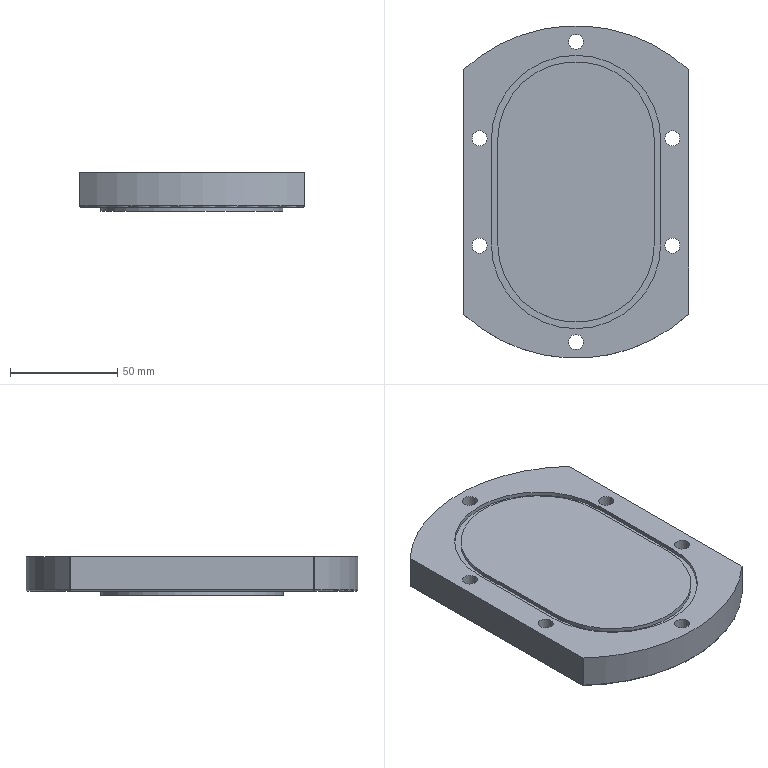Part | 1 solid | 52 faces | box 105 x 155 x 18 mm | volume 242328 mm3 | cylinder 24 | plane 17 | cone 6 | sphere 3 | torus 2 | commonest cylinder face diameters 7 x6 11 x6 1 x5 73 x2 79 x2 155 x2
STEP:
#1=CARTESIAN_POINT('',(52.5,-57.009,0.));
#2=VERTEX_POINT('',#1);
#3=CARTESIAN_POINT('',(-52.338,-57.158,0.));
#4=VERTEX_POINT('',#3);
#5=CARTESIAN_POINT('',(0.,0.,0.));
#6=DIRECTION('',(0.,0.,-1.));
#7=DIRECTION('',(-1.,0.,0.));
#8=AXIS2_PLACEMENT_3D('',#5,#6,#7);
#9=CIRCLE('',#8,77.5);
#10=EDGE_CURVE('',#2,#4,#9,.T.);
#11=ORIENTED_EDGE('',*,*,#10,.T.);
#12=CARTESIAN_POINT('',(-52.338,-57.158,-15.5));
#13=VERTEX_POINT('',#12);
#14=CARTESIAN_POINT('',(-52.338,-57.158,-16.));
#15=DIRECTION('',(0.,0.,1.));
#16=VECTOR('',#15,1000.);
#17=LINE('',#14,#16);
#18=EDGE_CURVE('',#4,#13,#17,.F.);
#19=ORIENTED_EDGE('',*,*,#18,.T.);
#20=CARTESIAN_POINT('',(52.5,-57.009,-15.5));
#21=VERTEX_POINT('',#20);
#22=CARTESIAN_POINT('',(0.,0.,-15.5));
#23=DIRECTION('',(0.,0.,-1.));
#24=DIRECTION('',(-1.,0.,0.));
#25=AXIS2_PLACEMENT_3D('',#22,#23,#24);
#26=CIRCLE('',#25,77.5);
#27=EDGE_CURVE('',#13,#21,#26,.F.);
#28=ORIENTED_EDGE('',*,*,#27,.T.);
#29=CARTESIAN_POINT('',(52.5,-57.009,-16.));
#30=DIRECTION('',(0.,0.,1.));
#31=VECTOR('',#30,1000.);
#32=LINE('',#29,#31);
#33=EDGE_CURVE('',#21,#2,#32,.T.);
#34=ORIENTED_EDGE('',*,*,#33,.T.);
#35=EDGE_LOOP('',(#11,#19,#28,#34));
#36=FACE_BOUND('',#35,.T.);
#37=CARTESIAN_POINT('',(0.,0.,-16.));
#38=DIRECTION('',(0.,0.,1.));
#39=DIRECTION('',(1.,0.,0.));
#40=AXIS2_PLACEMENT_3D('',#37,#38,#39);
#41=CYLINDRICAL_SURFACE('',#40,77.5);
#42=ADVANCED_FACE('',(#36),#41,.T.);
#43=CARTESIAN_POINT('',(-52.5,-56.789,0.));
#44=VERTEX_POINT('',#43);
#45=CARTESIAN_POINT('',(-52.5,56.789,0.));
#46=VERTEX_POINT('',#45);
#47=CARTESIAN_POINT('',(-52.5,-57.009,0.));
#48=DIRECTION('',(0.,1.,0.));
#49=VECTOR('',#48,1000.);
#50=LINE('',#47,#49);
#51=EDGE_CURVE('',#44,#46,#50,.T.);
#52=ORIENTED_EDGE('',*,*,#51,.T.);
#53=CARTESIAN_POINT('',(-52.5,56.789,-15.5));
#54=VERTEX_POINT('',#53);
#55=CARTESIAN_POINT('',(-52.5,56.789,-16.));
#56=DIRECTION('',(0.,0.,1.));
#57=VECTOR('',#56,1000.);
#58=LINE('',#55,#57);
#59=EDGE_CURVE('',#46,#54,#58,.F.);
#60=ORIENTED_EDGE('',*,*,#59,.T.);
#61=CARTESIAN_POINT('',(-52.5,-56.789,-15.5));
#62=VERTEX_POINT('',#61);
#63=CARTESIAN_POINT('',(-52.5,-57.009,-15.5));
#64=DIRECTION('',(0.,1.,0.));
#65=VECTOR('',#64,1000.);
#66=LINE('',#63,#65);
#67=EDGE_CURVE('',#54,#62,#66,.F.);
#68=ORIENTED_EDGE('',*,*,#67,.T.);
#69=CARTESIAN_POINT('',(-52.5,-56.789,-16.));
#70=DIRECTION('',(0.,0.,1.));
#71=VECTOR('',#70,1000.);
#72=LINE('',#69,#71);
#73=EDGE_CURVE('',#62,#44,#72,.T.);
#74=ORIENTED_EDGE('',*,*,#73,.T.);
#75=EDGE_LOOP('',(#52,#60,#68,#74));
#76=FACE_BOUND('',#75,.T.);
#77=CARTESIAN_POINT('',(-52.5,-57.009,-16.));
#78=DIRECTION('',(1.,0.,0.));
#79=DIRECTION('',(0.,0.,-1.));
#80=AXIS2_PLACEMENT_3D('',#77,#78,#79);
#81=PLANE('',#80);
#82=ADVANCED_FACE('',(#76),#81,.F.);
#83=CARTESIAN_POINT('',(-52.338,57.158,0.));
#84=VERTEX_POINT('',#83);
#85=CARTESIAN_POINT('',(52.338,57.158,0.));
#86=VERTEX_POINT('',#85);
#87=CARTESIAN_POINT('',(0.,0.,0.));
#88=DIRECTION('',(0.,0.,-1.));
#89=DIRECTION('',(-1.,0.,0.));
#90=AXIS2_PLACEMENT_3D('',#87,#88,#89);
#91=CIRCLE('',#90,77.5);
#92=EDGE_CURVE('',#84,#86,#91,.T.);
#93=ORIENTED_EDGE('',*,*,#92,.T.);
#94=CARTESIAN_POINT('',(52.338,57.158,-15.5));
#95=VERTEX_POINT('',#94);
#96=CARTESIAN_POINT('',(52.338,57.158,-16.));
#97=DIRECTION('',(0.,0.,1.));
#98=VECTOR('',#97,1000.);
#99=LINE('',#96,#98);
#100=EDGE_CURVE('',#86,#95,#99,.F.);
#101=ORIENTED_EDGE('',*,*,#100,.T.);
#102=CARTESIAN_POINT('',(-52.338,57.158,-15.5));
#103=VERTEX_POINT('',#102);
#104=CARTESIAN_POINT('',(0.,0.,-15.5));
#105=DIRECTION('',(0.,0.,-1.));
#106=DIRECTION('',(-1.,0.,0.));
#107=AXIS2_PLACEMENT_3D('',#104,#105,#106);
#108=CIRCLE('',#107,77.5);
#109=EDGE_CURVE('',#95,#103,#108,.F.);
#110=ORIENTED_EDGE('',*,*,#109,.T.);
#111=CARTESIAN_POINT('',(-52.338,57.158,-16.));
#112=DIRECTION('',(0.,0.,1.));
#113=VECTOR('',#112,1000.);
#114=LINE('',#111,#113);
#115=EDGE_CURVE('',#103,#84,#114,.T.);
#116=ORIENTED_EDGE('',*,*,#115,.T.);
#117=EDGE_LOOP('',(#93,#101,#110,#116));
#118=FACE_BOUND('',#117,.T.);
#119=CARTESIAN_POINT('',(0.,0.,-16.));
#120=DIRECTION('',(0.,0.,1.));
#121=DIRECTION('',(1.,0.,0.));
#122=AXIS2_PLACEMENT_3D('',#119,#120,#121);
#123=CYLINDRICAL_SURFACE('',#122,77.5);
#124=ADVANCED_FACE('',(#118),#123,.T.);
#125=CARTESIAN_POINT('',(52.5,56.789,-15.5));
#126=VERTEX_POINT('',#125);
#127=CARTESIAN_POINT('',(52.5,57.009,-15.5));
#128=DIRECTION('',(0.,-1.,0.));
#129=VECTOR('',#128,1000.);
#130=LINE('',#127,#129);
#131=EDGE_CURVE('',#21,#126,#130,.F.);
#132=ORIENTED_EDGE('',*,*,#131,.T.);
#133=CARTESIAN_POINT('',(52.5,56.789,0.));
#134=VERTEX_POINT('',#133);
#135=CARTESIAN_POINT('',(52.5,56.789,-16.));
#136=DIRECTION('',(0.,0.,1.));
#137=VECTOR('',#136,1000.);
#138=LINE('',#135,#137);
#139=EDGE_CURVE('',#126,#134,#138,.T.);
#140=ORIENTED_EDGE('',*,*,#139,.T.);
#141=CARTESIAN_POINT('',(52.5,57.009,0.));
#142=DIRECTION('',(0.,-1.,0.));
#143=VECTOR('',#142,1000.);
#144=LINE('',#141,#143);
#145=EDGE_CURVE('',#134,#2,#144,.T.);
#146=ORIENTED_EDGE('',*,*,#145,.T.);
#147=ORIENTED_EDGE('',*,*,#33,.F.);
#148=EDGE_LOOP('',(#132,#140,#146,#147));
#149=FACE_BOUND('',#148,.T.);
#150=CARTESIAN_POINT('',(52.5,57.009,-16.));
#151=DIRECTION('',(-1.,0.,0.));
#152=DIRECTION('',(0.,0.,1.));
#153=AXIS2_PLACEMENT_3D('',#150,#151,#152);
#154=PLANE('',#153);
#155=ADVANCED_FACE('',(#149),#154,.F.);
#156=CARTESIAN_POINT('',(-52.,-56.789,-16.));
#157=VERTEX_POINT('',#156);
#158=CARTESIAN_POINT('',(-52.,56.789,-16.));
#159=VERTEX_POINT('',#158);
#160=CARTESIAN_POINT('',(-52.,57.009,-16.));
#161=DIRECTION('',(0.,1.,0.));
#162=VECTOR('',#161,1000.);
#163=LINE('',#160,#162);
#164=EDGE_CURVE('',#157,#159,#163,.T.);
#165=ORIENTED_EDGE('',*,*,#164,.T.);
#166=CARTESIAN_POINT('',(52.,56.789,-16.));
#167=VERTEX_POINT('',#166);
#168=CARTESIAN_POINT('',(0.,0.,-16.));
#169=DIRECTION('',(0.,0.,-1.));
#170=DIRECTION('',(-1.,0.,0.));
#171=AXIS2_PLACEMENT_3D('',#168,#169,#170);
#172=CIRCLE('',#171,77.);
#173=EDGE_CURVE('',#159,#167,#172,.T.);
#174=ORIENTED_EDGE('',*,*,#173,.T.);
#175=CARTESIAN_POINT('',(52.,-56.789,-16.));
#176=VERTEX_POINT('',#175);
#177=CARTESIAN_POINT('',(52.,-57.009,-16.));
#178=DIRECTION('',(0.,-1.,0.));
#179=VECTOR('',#178,1000.);
#180=LINE('',#177,#179);
#181=EDGE_CURVE('',#167,#176,#180,.T.);
#182=ORIENTED_EDGE('',*,*,#181,.T.);
#183=CARTESIAN_POINT('',(0.,0.,-16.));
#184=DIRECTION('',(0.,0.,-1.));
#185=DIRECTION('',(-1.,0.,0.));
#186=AXIS2_PLACEMENT_3D('',#183,#184,#185);
#187=CIRCLE('',#186,77.);
#188=EDGE_CURVE('',#176,#157,#187,.T.);
#189=ORIENTED_EDGE('',*,*,#188,.T.);
#190=EDGE_LOOP('',(#165,#174,#182,#189));
#191=FACE_BOUND('',#190,.T.);
#192=CARTESIAN_POINT('',(-5.525,70.,-16.));
#193=VERTEX_POINT('',#192);
#194=CARTESIAN_POINT('',(0.,70.,-16.));
#195=DIRECTION('',(0.,0.,-1.));
#196=DIRECTION('',(-1.,0.,0.));
#197=AXIS2_PLACEMENT_3D('',#194,#195,#196);
#198=CIRCLE('',#197,5.525);
#199=EDGE_CURVE('',#193,#193,#198,.T.);
#200=ORIENTED_EDGE('',*,*,#199,.F.);
#201=EDGE_LOOP('',(#200));
#202=FACE_BOUND('',#201,.T.);
#203=CARTESIAN_POINT('',(39.475,25.,-16.));
#204=VERTEX_POINT('',#203);
#205=CARTESIAN_POINT('',(45.,25.,-16.));
#206=DIRECTION('',(0.,0.,-1.));
#207=DIRECTION('',(-1.,0.,0.));
#208=AXIS2_PLACEMENT_3D('',#205,#206,#207);
#209=CIRCLE('',#208,5.525);
#210=EDGE_CURVE('',#204,#204,#209,.T.);
#211=ORIENTED_EDGE('',*,*,#210,.F.);
#212=EDGE_LOOP('',(#211));
#213=FACE_BOUND('',#212,.T.);
#214=CARTESIAN_POINT('',(-50.525,25.,-16.));
#215=VERTEX_POINT('',#214);
#216=CARTESIAN_POINT('',(-45.,25.,-16.));
#217=DIRECTION('',(0.,0.,-1.));
#218=DIRECTION('',(-1.,0.,0.));
#219=AXIS2_PLACEMENT_3D('',#216,#217,#218);
#220=CIRCLE('',#219,5.525);
#221=EDGE_CURVE('',#215,#215,#220,.T.);
#222=ORIENTED_EDGE('',*,*,#221,.F.);
#223=EDGE_LOOP('',(#222));
#224=FACE_BOUND('',#223,.T.);
#225=CARTESIAN_POINT('',(-50.525,-25.,-16.));
#226=VERTEX_POINT('',#225);
#227=CARTESIAN_POINT('',(-45.,-25.,-16.));
#228=DIRECTION('',(0.,0.,-1.));
#229=DIRECTION('',(-1.,0.,0.));
#230=AXIS2_PLACEMENT_3D('',#227,#228,#229);
#231=CIRCLE('',#230,5.525);
#232=EDGE_CURVE('',#226,#226,#231,.T.);
#233=ORIENTED_EDGE('',*,*,#232,.F.);
#234=EDGE_LOOP('',(#233));
#235=FACE_BOUND('',#234,.T.);
#236=CARTESIAN_POINT('',(39.475,-25.,-16.));
#237=VERTEX_POINT('',#236);
#238=CARTESIAN_POINT('',(45.,-25.,-16.));
#239=DIRECTION('',(0.,0.,-1.));
#240=DIRECTION('',(-1.,0.,0.));
#241=AXIS2_PLACEMENT_3D('',#238,#239,#240);
#242=CIRCLE('',#241,5.525);
#243=EDGE_CURVE('',#237,#237,#242,.T.);
#244=ORIENTED_EDGE('',*,*,#243,.F.);
#245=EDGE_LOOP('',(#244));
#246=FACE_BOUND('',#245,.T.);
#247=CARTESIAN_POINT('',(-5.525,-70.,-16.));
#248=VERTEX_POINT('',#247);
#249=CARTESIAN_POINT('',(0.,-70.,-16.));
#250=DIRECTION('',(0.,0.,-1.));
#251=DIRECTION('',(-1.,0.,0.));
#252=AXIS2_PLACEMENT_3D('',#249,#250,#251);
#253=CIRCLE('',#252,5.525);
#254=EDGE_CURVE('',#248,#248,#253,.T.);
#255=ORIENTED_EDGE('',*,*,#254,.F.);
#256=EDGE_LOOP('',(#255));
#257=FACE_BOUND('',#256,.T.);
#258=CARTESIAN_POINT('',(-42.5,0.,-16.));
#259=VERTEX_POINT('',#258);
#260=CARTESIAN_POINT('',(0.,0.,-16.));
#261=DIRECTION('',(0.,0.,-1.));
#262=DIRECTION('',(-1.,0.,0.));
#263=AXIS2_PLACEMENT_3D('',#260,#261,#262);
#264=CIRCLE('',#263,42.5);
#265=EDGE_CURVE('',#259,#259,#264,.T.);
#266=ORIENTED_EDGE('',*,*,#265,.F.);
#267=EDGE_LOOP('',(#266));
#268=FACE_BOUND('',#267,.T.);
#269=CARTESIAN_POINT('',(0.,0.,-16.));
#270=DIRECTION('',(0.,0.,-1.));
#271=DIRECTION('',(-1.,0.,0.));
#272=AXIS2_PLACEMENT_3D('',#269,#270,#271);
#273=PLANE('',#272);
#274=ADVANCED_FACE('',(#191,#202,#213,#224,#235,#246,#257,#268),#273,.T.);
#275=CARTESIAN_POINT('',(-39.5,24.25,0.));
#276=VERTEX_POINT('',#275);
#277=CARTESIAN_POINT('',(-39.5,-24.25,0.));
#278=VERTEX_POINT('',#277);
#279=CARTESIAN_POINT('',(-39.5,24.25,0.));
#280=DIRECTION('',(0.,-1.,0.));
#281=VECTOR('',#280,1000.);
#282=LINE('',#279,#281);
#283=EDGE_CURVE('',#276,#278,#282,.T.);
#284=ORIENTED_EDGE('',*,*,#283,.F.);
#285=CARTESIAN_POINT('',(39.5,24.25,0.));
#286=VERTEX_POINT('',#285);
#287=CARTESIAN_POINT('',(0.,24.25,0.));
#288=DIRECTION('',(0.,0.,1.));
#289=DIRECTION('',(1.,0.,0.));
#290=AXIS2_PLACEMENT_3D('',#287,#288,#289);
#291=CIRCLE('',#290,39.5);
#292=EDGE_CURVE('',#286,#276,#291,.T.);
#293=ORIENTED_EDGE('',*,*,#292,.F.);
#294=CARTESIAN_POINT('',(39.5,-24.25,0.));
#295=VERTEX_POINT('',#294);
#296=CARTESIAN_POINT('',(39.5,24.25,0.));
#297=DIRECTION('',(0.,1.,0.));
#298=VECTOR('',#297,1000.);
#299=LINE('',#296,#298);
#300=EDGE_CURVE('',#295,#286,#299,.T.);
#301=ORIENTED_EDGE('',*,*,#300,.F.);
#302=CARTESIAN_POINT('',(0.,-24.25,0.));
#303=DIRECTION('',(0.,0.,1.));
#304=DIRECTION('',(1.,0.,0.));
#305=AXIS2_PLACEMENT_3D('',#302,#303,#304);
#306=CIRCLE('',#305,39.5);
#307=EDGE_CURVE('',#278,#295,#306,.T.);
#308=ORIENTED_EDGE('',*,*,#307,.F.);
#309=EDGE_LOOP('',(#284,#293,#301,#308));
#310=FACE_BOUND('',#309,.T.);
#311=CARTESIAN_POINT('',(-3.5,70.,0.));
#312=VERTEX_POINT('',#311);
#313=CARTESIAN_POINT('',(0.,70.,0.));
#314=DIRECTION('',(0.,0.,-1.));
#315=DIRECTION('',(-1.,0.,0.));
#316=AXIS2_PLACEMENT_3D('',#313,#314,#315);
#317=CIRCLE('',#316,3.5);
#318=EDGE_CURVE('',#312,#312,#317,.T.);
#319=ORIENTED_EDGE('',*,*,#318,.T.);
#320=EDGE_LOOP('',(#319));
#321=FACE_BOUND('',#320,.T.);
#322=CARTESIAN_POINT('',(41.5,25.,0.));
#323=VERTEX_POINT('',#322);
#324=CARTESIAN_POINT('',(45.,25.,0.));
#325=DIRECTION('',(0.,0.,-1.));
#326=DIRECTION('',(-1.,0.,0.));
#327=AXIS2_PLACEMENT_3D('',#324,#325,#326);
#328=CIRCLE('',#327,3.5);
#329=EDGE_CURVE('',#323,#323,#328,.T.);
#330=ORIENTED_EDGE('',*,*,#329,.T.);
#331=EDGE_LOOP('',(#330));
#332=FACE_BOUND('',#331,.T.);
#333=CARTESIAN_POINT('',(-48.5,25.,0.));
#334=VERTEX_POINT('',#333);
#335=CARTESIAN_POINT('',(-45.,25.,0.));
#336=DIRECTION('',(0.,0.,-1.));
#337=DIRECTION('',(-1.,0.,0.));
#338=AXIS2_PLACEMENT_3D('',#335,#336,#337);
#339=CIRCLE('',#338,3.5);
#340=EDGE_CURVE('',#334,#334,#339,.T.);
#341=ORIENTED_EDGE('',*,*,#340,.T.);
#342=EDGE_LOOP('',(#341));
#343=FACE_BOUND('',#342,.T.);
#344=CARTESIAN_POINT('',(-48.5,-25.,0.));
#345=VERTEX_POINT('',#344);
#346=CARTESIAN_POINT('',(-45.,-25.,0.));
#347=DIRECTION('',(0.,0.,-1.));
#348=DIRECTION('',(-1.,0.,0.));
#349=AXIS2_PLACEMENT_3D('',#346,#347,#348);
#350=CIRCLE('',#349,3.5);
#351=EDGE_CURVE('',#345,#345,#350,.T.);
#352=ORIENTED_EDGE('',*,*,#351,.T.);
#353=EDGE_LOOP('',(#352));
#354=FACE_BOUND('',#353,.T.);
#355=CARTESIAN_POINT('',(41.5,-25.,0.));
#356=VERTEX_POINT('',#355);
#357=CARTESIAN_POINT('',(45.,-25.,0.));
#358=DIRECTION('',(0.,0.,-1.));
#359=DIRECTION('',(-1.,0.,0.));
#360=AXIS2_PLACEMENT_3D('',#357,#358,#359);
#361=CIRCLE('',#360,3.5);
#362=EDGE_CURVE('',#356,#356,#361,.T.);
#363=ORIENTED_EDGE('',*,*,#362,.T.);
#364=EDGE_LOOP('',(#363));
#365=FACE_BOUND('',#364,.T.);
#366=CARTESIAN_POINT('',(-3.5,-70.,0.));
#367=VERTEX_POINT('',#366);
#368=CARTESIAN_POINT('',(0.,-70.,0.));
#369=DIRECTION('',(0.,0.,-1.));
#370=DIRECTION('',(-1.,0.,0.));
#371=AXIS2_PLACEMENT_3D('',#368,#369,#370);
#372=CIRCLE('',#371,3.5);
#373=EDGE_CURVE('',#367,#367,#372,.T.);
#374=ORIENTED_EDGE('',*,*,#373,.T.);
#375=EDGE_LOOP('',(#374));
#376=FACE_BOUND('',#375,.T.);
#377=ORIENTED_EDGE('',*,*,#145,.F.);
#378=CARTESIAN_POINT('',(52.,56.789,0.));
#379=DIRECTION('',(0.,0.,-1.));
#380=DIRECTION('',(-1.,0.,0.));
#381=AXIS2_PLACEMENT_3D('',#378,#379,#380);
#382=CIRCLE('',#381,0.5);
#383=EDGE_CURVE('',#134,#86,#382,.F.);
#384=ORIENTED_EDGE('',*,*,#383,.T.);
#385=ORIENTED_EDGE('',*,*,#92,.F.);
#386=CARTESIAN_POINT('',(-52.,56.789,0.));
#387=DIRECTION('',(0.,0.,-1.));
#388=DIRECTION('',(-1.,0.,0.));
#389=AXIS2_PLACEMENT_3D('',#386,#387,#388);
#390=CIRCLE('',#389,0.5);
#391=EDGE_CURVE('',#84,#46,#390,.F.);
#392=ORIENTED_EDGE('',*,*,#391,.T.);
#393=ORIENTED_EDGE('',*,*,#51,.F.);
#394=CARTESIAN_POINT('',(-52.,-56.789,0.));
#395=DIRECTION('',(0.,0.,-1.));
#396=DIRECTION('',(-1.,0.,0.));
#397=AXIS2_PLACEMENT_3D('',#394,#395,#396);
#398=CIRCLE('',#397,0.5);
#399=EDGE_CURVE('',#44,#4,#398,.F.);
#400=ORIENTED_EDGE('',*,*,#399,.T.);
#401=ORIENTED_EDGE('',*,*,#10,.F.);
#402=EDGE_LOOP('',(#377,#384,#385,#392,#393,#400,#401));
#403=FACE_BOUND('',#402,.T.);
#404=CARTESIAN_POINT('',(0.,0.,0.));
#405=DIRECTION('',(0.,0.,-1.));
#406=DIRECTION('',(-1.,0.,0.));
#407=AXIS2_PLACEMENT_3D('',#404,#405,#406);
#408=PLANE('',#407);
#409=ADVANCED_FACE('',(#310,#321,#332,#343,#354,#365,#376,#403),#408,.F.);
#410=CARTESIAN_POINT('',(-42.5,0.,-18.));
#411=VERTEX_POINT('',#410);
#412=CARTESIAN_POINT('',(0.,0.,-18.));
#413=DIRECTION('',(0.,0.,-1.));
#414=DIRECTION('',(-1.,0.,0.));
#415=AXIS2_PLACEMENT_3D('',#412,#413,#414);
#416=CIRCLE('',#415,42.5);
#417=EDGE_CURVE('',#411,#411,#416,.T.);
#418=ORIENTED_EDGE('',*,*,#417,.F.);
#419=EDGE_LOOP('',(#418));
#420=FACE_BOUND('',#419,.T.);
#421=ORIENTED_EDGE('',*,*,#265,.T.);
#422=EDGE_LOOP('',(#421));
#423=FACE_BOUND('',#422,.T.);
#424=CARTESIAN_POINT('',(0.,0.,-18.));
#425=DIRECTION('',(0.,0.,1.));
#426=DIRECTION('',(1.,0.,0.));
#427=AXIS2_PLACEMENT_3D('',#424,#425,#426);
#428=CYLINDRICAL_SURFACE('',#427,42.5);
#429=ADVANCED_FACE('',(#420,#423),#428,.T.);
#430=ORIENTED_EDGE('',*,*,#417,.T.);
#431=EDGE_LOOP('',(#430));
#432=FACE_BOUND('',#431,.T.);
#433=CARTESIAN_POINT('',(0.,0.,-18.));
#434=DIRECTION('',(0.,0.,-1.));
#435=DIRECTION('',(-1.,0.,0.));
#436=AXIS2_PLACEMENT_3D('',#433,#434,#435);
#437=PLANE('',#436);
#438=ADVANCED_FACE('',(#432),#437,.T.);
#439=CARTESIAN_POINT('',(-3.5,-70.,-9.2));
#440=VERTEX_POINT('',#439);
#441=CARTESIAN_POINT('',(0.,-70.,-9.2));
#442=DIRECTION('',(0.,0.,-1.));
#443=DIRECTION('',(-1.,0.,0.));
#444=AXIS2_PLACEMENT_3D('',#441,#442,#443);
#445=CIRCLE('',#444,3.5);
#446=EDGE_CURVE('',#440,#440,#445,.T.);
#447=ORIENTED_EDGE('',*,*,#446,.T.);
#448=EDGE_LOOP('',(#447));
#449=FACE_BOUND('',#448,.T.);
#450=ORIENTED_EDGE('',*,*,#373,.F.);
#451=EDGE_LOOP('',(#450));
#452=FACE_BOUND('',#451,.T.);
#453=CARTESIAN_POINT('',(0.,-70.,-16.));
#454=DIRECTION('',(0.,0.,-1.));
#455=DIRECTION('',(-1.,0.,0.));
#456=AXIS2_PLACEMENT_3D('',#453,#454,#455);
#457=CYLINDRICAL_SURFACE('',#456,3.5);
#458=ADVANCED_FACE('',(#449,#452),#457,.F.);
#459=ORIENTED_EDGE('',*,*,#446,.F.);
#460=EDGE_LOOP('',(#459));
#461=FACE_BOUND('',#460,.T.);
#462=CARTESIAN_POINT('',(-5.5,-70.,-9.2));
#463=VERTEX_POINT('',#462);
#464=CARTESIAN_POINT('',(0.,-70.,-9.2));
#465=DIRECTION('',(0.,0.,-1.));
#466=DIRECTION('',(-1.,0.,0.));
#467=AXIS2_PLACEMENT_3D('',#464,#465,#466);
#468=CIRCLE('',#467,5.5);
#469=EDGE_CURVE('',#463,#463,#468,.T.);
#470=ORIENTED_EDGE('',*,*,#469,.T.);
#471=EDGE_LOOP('',(#470));
#472=FACE_BOUND('',#471,.T.);
#473=CARTESIAN_POINT('',(-3.5,-70.,-9.2));
#474=DIRECTION('',(0.,0.,1.));
#475=DIRECTION('',(1.,0.,0.));
#476=AXIS2_PLACEMENT_3D('',#473,#474,#475);
#477=PLANE('',#476);
#478=ADVANCED_FACE('',(#461,#472),#477,.F.);
#479=ORIENTED_EDGE('',*,*,#469,.F.);
#480=EDGE_LOOP('',(#479));
#481=FACE_BOUND('',#480,.T.);
#482=CARTESIAN_POINT('',(-5.5,-70.,-15.975));
#483=VERTEX_POINT('',#482);
#484=CARTESIAN_POINT('',(0.,-70.,-15.975));
#485=DIRECTION('',(0.,0.,-1.));
#486=DIRECTION('',(-1.,0.,0.));
#487=AXIS2_PLACEMENT_3D('',#484,#485,#486);
#488=CIRCLE('',#487,5.5);
#489=EDGE_CURVE('',#483,#483,#488,.T.);
#490=ORIENTED_EDGE('',*,*,#489,.T.);
#491=EDGE_LOOP('',(#490));
#492=FACE_BOUND('',#491,.T.);
#493=CARTESIAN_POINT('',(0.,-70.,-16.));
#494=DIRECTION('',(0.,0.,-1.));
#495=DIRECTION('',(-1.,0.,0.));
#496=AXIS2_PLACEMENT_3D('',#493,#494,#495);
#497=CYLINDRICAL_SURFACE('',#496,5.5);
#498=ADVANCED_FACE('',(#481,#492),#497,.F.);
#499=ORIENTED_EDGE('',*,*,#489,.F.);
#500=EDGE_LOOP('',(#499));
#501=FACE_BOUND('',#500,.T.);
#502=ORIENTED_EDGE('',*,*,#254,.T.);
#503=EDGE_LOOP('',(#502));
#504=FACE_BOUND('',#503,.T.);
#505=CARTESIAN_POINT('',(0.,-70.,-16.));
#506=DIRECTION('',(0.,0.,-1.));
#507=DIRECTION('',(-1.,0.,0.));
#508=AXIS2_PLACEMENT_3D('',#505,#506,#507);
#509=CONICAL_SURFACE('',#508,5.525,0.7854);
#510=ADVANCED_FACE('',(#501,#504),#509,.F.);
#511=CARTESIAN_POINT('',(41.5,-25.,-9.2));
#512=VERTEX_POINT('',#511);
#513=CARTESIAN_POINT('',(45.,-25.,-9.2));
#514=DIRECTION('',(0.,0.,-1.));
#515=DIRECTION('',(-1.,0.,0.));
#516=AXIS2_PLACEMENT_3D('',#513,#514,#515);
#517=CIRCLE('',#516,3.5);
#518=EDGE_CURVE('',#512,#512,#517,.T.);
#519=ORIENTED_EDGE('',*,*,#518,.T.);
#520=EDGE_LOOP('',(#519));
#521=FACE_BOUND('',#520,.T.);
#522=ORIENTED_EDGE('',*,*,#362,.F.);
#523=EDGE_LOOP('',(#522));
#524=FACE_BOUND('',#523,.T.);
#525=CARTESIAN_POINT('',(45.,-25.,-16.));
#526=DIRECTION('',(0.,0.,-1.));
#527=DIRECTION('',(-1.,0.,0.));
#528=AXIS2_PLACEMENT_3D('',#525,#526,#527);
#529=CYLINDRICAL_SURFACE('',#528,3.5);
#530=ADVANCED_FACE('',(#521,#524),#529,.F.);
#531=ORIENTED_EDGE('',*,*,#518,.F.);
#532=EDGE_LOOP('',(#531));
#533=FACE_BOUND('',#532,.T.);
#534=CARTESIAN_POINT('',(39.5,-25.,-9.2));
#535=VERTEX_POINT('',#534);
#536=CARTESIAN_POINT('',(45.,-25.,-9.2));
#537=DIRECTION('',(0.,0.,-1.));
#538=DIRECTION('',(-1.,0.,0.));
#539=AXIS2_PLACEMENT_3D('',#536,#537,#538);
#540=CIRCLE('',#539,5.5);
#541=EDGE_CURVE('',#535,#535,#540,.T.);
#542=ORIENTED_EDGE('',*,*,#541,.T.);
#543=EDGE_LOOP('',(#542));
#544=FACE_BOUND('',#543,.T.);
#545=CARTESIAN_POINT('',(41.5,-25.,-9.2));
#546=DIRECTION('',(0.,0.,1.));
#547=DIRECTION('',(1.,0.,0.));
#548=AXIS2_PLACEMENT_3D('',#545,#546,#547);
#549=PLANE('',#548);
#550=ADVANCED_FACE('',(#533,#544),#549,.F.);
#551=ORIENTED_EDGE('',*,*,#541,.F.);
#552=EDGE_LOOP('',(#551));
#553=FACE_BOUND('',#552,.T.);
#554=CARTESIAN_POINT('',(39.5,-25.,-15.975));
#555=VERTEX_POINT('',#554);
#556=CARTESIAN_POINT('',(45.,-25.,-15.975));
#557=DIRECTION('',(0.,0.,-1.));
#558=DIRECTION('',(-1.,0.,0.));
#559=AXIS2_PLACEMENT_3D('',#556,#557,#558);
#560=CIRCLE('',#559,5.5);
#561=EDGE_CURVE('',#555,#555,#560,.T.);
#562=ORIENTED_EDGE('',*,*,#561,.T.);
#563=EDGE_LOOP('',(#562));
#564=FACE_BOUND('',#563,.T.);
#565=CARTESIAN_POINT('',(45.,-25.,-16.));
#566=DIRECTION('',(0.,0.,-1.));
#567=DIRECTION('',(-1.,0.,0.));
#568=AXIS2_PLACEMENT_3D('',#565,#566,#567);
#569=CYLINDRICAL_SURFACE('',#568,5.5);
#570=ADVANCED_FACE('',(#553,#564),#569,.F.);
#571=ORIENTED_EDGE('',*,*,#561,.F.);
#572=EDGE_LOOP('',(#571));
#573=FACE_BOUND('',#572,.T.);
#574=ORIENTED_EDGE('',*,*,#243,.T.);
#575=EDGE_LOOP('',(#574));
#576=FACE_BOUND('',#575,.T.);
#577=CARTESIAN_POINT('',(45.,-25.,-16.));
#578=DIRECTION('',(0.,0.,-1.));
#579=DIRECTION('',(-1.,0.,0.));
#580=AXIS2_PLACEMENT_3D('',#577,#578,#579);
#581=CONICAL_SURFACE('',#580,5.525,0.7854);
#582=ADVANCED_FACE('',(#573,#576),#581,.F.);
#583=CARTESIAN_POINT('',(-48.5,-25.,-9.2));
#584=VERTEX_POINT('',#583);
#585=CARTESIAN_POINT('',(-45.,-25.,-9.2));
#586=DIRECTION('',(0.,0.,-1.));
#587=DIRECTION('',(-1.,0.,0.));
#588=AXIS2_PLACEMENT_3D('',#585,#586,#587);
#589=CIRCLE('',#588,3.5);
#590=EDGE_CURVE('',#584,#584,#589,.T.);
#591=ORIENTED_EDGE('',*,*,#590,.T.);
#592=EDGE_LOOP('',(#591));
#593=FACE_BOUND('',#592,.T.);
#594=ORIENTED_EDGE('',*,*,#351,.F.);
#595=EDGE_LOOP('',(#594));
#596=FACE_BOUND('',#595,.T.);
#597=CARTESIAN_POINT('',(-45.,-25.,-16.));
#598=DIRECTION('',(0.,0.,-1.));
#599=DIRECTION('',(-1.,0.,0.));
#600=AXIS2_PLACEMENT_3D('',#597,#598,#599);
#601=CYLINDRICAL_SURFACE('',#600,3.5);
#602=ADVANCED_FACE('',(#593,#596),#601,.F.);
#603=ORIENTED_EDGE('',*,*,#590,.F.);
#604=EDGE_LOOP('',(#603));
#605=FACE_BOUND('',#604,.T.);
#606=CARTESIAN_POINT('',(-50.5,-25.,-9.2));
#607=VERTEX_POINT('',#606);
#608=CARTESIAN_POINT('',(-45.,-25.,-9.2));
#609=DIRECTION('',(0.,0.,-1.));
#610=DIRECTION('',(-1.,0.,0.));
#611=AXIS2_PLACEMENT_3D('',#608,#609,#610);
#612=CIRCLE('',#611,5.5);
#613=EDGE_CURVE('',#607,#607,#612,.T.);
#614=ORIENTED_EDGE('',*,*,#613,.T.);
#615=EDGE_LOOP('',(#614));
#616=FACE_BOUND('',#615,.T.);
#617=CARTESIAN_POINT('',(-48.5,-25.,-9.2));
#618=DIRECTION('',(0.,0.,1.));
#619=DIRECTION('',(1.,0.,0.));
#620=AXIS2_PLACEMENT_3D('',#617,#618,#619);
#621=PLANE('',#620);
#622=ADVANCED_FACE('',(#605,#616),#621,.F.);
#623=ORIENTED_EDGE('',*,*,#613,.F.);
#624=EDGE_LOOP('',(#623));
#625=FACE_BOUND('',#624,.T.);
#626=CARTESIAN_POINT('',(-50.5,-25.,-15.975));
#627=VERTEX_POINT('',#626);
#628=CARTESIAN_POINT('',(-45.,-25.,-15.975));
#629=DIRECTION('',(0.,0.,-1.));
#630=DIRECTION('',(-1.,0.,0.));
#631=AXIS2_PLACEMENT_3D('',#628,#629,#630);
#632=CIRCLE('',#631,5.5);
#633=EDGE_CURVE('',#627,#627,#632,.T.);
#634=ORIENTED_EDGE('',*,*,#633,.T.);
#635=EDGE_LOOP('',(#634));
#636=FACE_BOUND('',#635,.T.);
#637=CARTESIAN_POINT('',(-45.,-25.,-16.));
#638=DIRECTION('',(0.,0.,-1.));
#639=DIRECTION('',(-1.,0.,0.));
#640=AXIS2_PLACEMENT_3D('',#637,#638,#639);
#641=CYLINDRICAL_SURFACE('',#640,5.5);
#642=ADVANCED_FACE('',(#625,#636),#641,.F.);
#643=ORIENTED_EDGE('',*,*,#633,.F.);
#644=EDGE_LOOP('',(#643));
#645=FACE_BOUND('',#644,.T.);
#646=ORIENTED_EDGE('',*,*,#232,.T.);
#647=EDGE_LOOP('',(#646));
#648=FACE_BOUND('',#647,.T.);
#649=CARTESIAN_POINT('',(-45.,-25.,-16.));
#650=DIRECTION('',(0.,0.,-1.));
#651=DIRECTION('',(-1.,0.,0.));
#652=AXIS2_PLACEMENT_3D('',#649,#650,#651);
#653=CONICAL_SURFACE('',#652,5.525,0.7854);
#654=ADVANCED_FACE('',(#645,#648),#653,.F.);
#655=CARTESIAN_POINT('',(-48.5,25.,-9.2));
#656=VERTEX_POINT('',#655);
#657=CARTESIAN_POINT('',(-45.,25.,-9.2));
#658=DIRECTION('',(0.,0.,-1.));
#659=DIRECTION('',(-1.,0.,0.));
#660=AXIS2_PLACEMENT_3D('',#657,#658,#659);
#661=CIRCLE('',#660,3.5);
#662=EDGE_CURVE('',#656,#656,#661,.T.);
#663=ORIENTED_EDGE('',*,*,#662,.T.);
#664=EDGE_LOOP('',(#663));
#665=FACE_BOUND('',#664,.T.);
#666=ORIENTED_EDGE('',*,*,#340,.F.);
#667=EDGE_LOOP('',(#666));
#668=FACE_BOUND('',#667,.T.);
#669=CARTESIAN_POINT('',(-45.,25.,-16.));
#670=DIRECTION('',(0.,0.,-1.));
#671=DIRECTION('',(-1.,0.,0.));
#672=AXIS2_PLACEMENT_3D('',#669,#670,#671);
#673=CYLINDRICAL_SURFACE('',#672,3.5);
#674=ADVANCED_FACE('',(#665,#668),#673,.F.);
#675=ORIENTED_EDGE('',*,*,#662,.F.);
#676=EDGE_LOOP('',(#675));
#677=FACE_BOUND('',#676,.T.);
#678=CARTESIAN_POINT('',(-50.5,25.,-9.2));
#679=VERTEX_POINT('',#678);
#680=CARTESIAN_POINT('',(-45.,25.,-9.2));
#681=DIRECTION('',(0.,0.,-1.));
#682=DIRECTION('',(-1.,0.,0.));
#683=AXIS2_PLACEMENT_3D('',#680,#681,#682);
#684=CIRCLE('',#683,5.5);
#685=EDGE_CURVE('',#679,#679,#684,.T.);
#686=ORIENTED_EDGE('',*,*,#685,.T.);
#687=EDGE_LOOP('',(#686));
#688=FACE_BOUND('',#687,.T.);
#689=CARTESIAN_POINT('',(-48.5,25.,-9.2));
#690=DIRECTION('',(0.,0.,1.));
#691=DIRECTION('',(1.,0.,0.));
#692=AXIS2_PLACEMENT_3D('',#689,#690,#691);
#693=PLANE('',#692);
#694=ADVANCED_FACE('',(#677,#688),#693,.F.);
#695=ORIENTED_EDGE('',*,*,#685,.F.);
#696=EDGE_LOOP('',(#695));
#697=FACE_BOUND('',#696,.T.);
#698=CARTESIAN_POINT('',(-50.5,25.,-15.975));
#699=VERTEX_POINT('',#698);
#700=CARTESIAN_POINT('',(-45.,25.,-15.975));
#701=DIRECTION('',(0.,0.,-1.));
#702=DIRECTION('',(-1.,0.,0.));
#703=AXIS2_PLACEMENT_3D('',#700,#701,#702);
#704=CIRCLE('',#703,5.5);
#705=EDGE_CURVE('',#699,#699,#704,.T.);
#706=ORIENTED_EDGE('',*,*,#705,.T.);
#707=EDGE_LOOP('',(#706));
#708=FACE_BOUND('',#707,.T.);
#709=CARTESIAN_POINT('',(-45.,25.,-16.));
#710=DIRECTION('',(0.,0.,-1.));
#711=DIRECTION('',(-1.,0.,0.));
#712=AXIS2_PLACEMENT_3D('',#709,#710,#711);
#713=CYLINDRICAL_SURFACE('',#712,5.5);
#714=ADVANCED_FACE('',(#697,#708),#713,.F.);
#715=ORIENTED_EDGE('',*,*,#705,.F.);
#716=EDGE_LOOP('',(#715));
#717=FACE_BOUND('',#716,.T.);
#718=ORIENTED_EDGE('',*,*,#221,.T.);
#719=EDGE_LOOP('',(#718));
#720=FACE_BOUND('',#719,.T.);
#721=CARTESIAN_POINT('',(-45.,25.,-16.));
#722=DIRECTION('',(0.,0.,-1.));
#723=DIRECTION('',(-1.,0.,0.));
#724=AXIS2_PLACEMENT_3D('',#721,#722,#723);
#725=CONICAL_SURFACE('',#724,5.525,0.7854);
#726=ADVANCED_FACE('',(#717,#720),#725,.F.);
#727=CARTESIAN_POINT('',(41.5,25.,-9.2));
#728=VERTEX_POINT('',#727);
#729=CARTESIAN_POINT('',(45.,25.,-9.2));
#730=DIRECTION('',(0.,0.,-1.));
#731=DIRECTION('',(-1.,0.,0.));
#732=AXIS2_PLACEMENT_3D('',#729,#730,#731);
#733=CIRCLE('',#732,3.5);
#734=EDGE_CURVE('',#728,#728,#733,.T.);
#735=ORIENTED_EDGE('',*,*,#734,.T.);
#736=EDGE_LOOP('',(#735));
#737=FACE_BOUND('',#736,.T.);
#738=ORIENTED_EDGE('',*,*,#329,.F.);
#739=EDGE_LOOP('',(#738));
#740=FACE_BOUND('',#739,.T.);
#741=CARTESIAN_POINT('',(45.,25.,-16.));
#742=DIRECTION('',(0.,0.,-1.));
#743=DIRECTION('',(-1.,0.,0.));
#744=AXIS2_PLACEMENT_3D('',#741,#742,#743);
#745=CYLINDRICAL_SURFACE('',#744,3.5);
#746=ADVANCED_FACE('',(#737,#740),#745,.F.);
#747=ORIENTED_EDGE('',*,*,#734,.F.);
#748=EDGE_LOOP('',(#747));
#749=FACE_BOUND('',#748,.T.);
#750=CARTESIAN_POINT('',(39.5,25.,-9.2));
#751=VERTEX_POINT('',#750);
#752=CARTESIAN_POINT('',(45.,25.,-9.2));
#753=DIRECTION('',(0.,0.,-1.));
#754=DIRECTION('',(-1.,0.,0.));
#755=AXIS2_PLACEMENT_3D('',#752,#753,#754);
#756=CIRCLE('',#755,5.5);
#757=EDGE_CURVE('',#751,#751,#756,.T.);
#758=ORIENTED_EDGE('',*,*,#757,.T.);
#759=EDGE_LOOP('',(#758));
#760=FACE_BOUND('',#759,.T.);
#761=CARTESIAN_POINT('',(41.5,25.,-9.2));
#762=DIRECTION('',(0.,0.,1.));
#763=DIRECTION('',(1.,0.,0.));
#764=AXIS2_PLACEMENT_3D('',#761,#762,#763);
#765=PLANE('',#764);
#766=ADVANCED_FACE('',(#749,#760),#765,.F.);
#767=ORIENTED_EDGE('',*,*,#757,.F.);
#768=EDGE_LOOP('',(#767));
#769=FACE_BOUND('',#768,.T.);
#770=CARTESIAN_POINT('',(39.5,25.,-15.975));
#771=VERTEX_POINT('',#770);
#772=CARTESIAN_POINT('',(45.,25.,-15.975));
#773=DIRECTION('',(0.,0.,-1.));
#774=DIRECTION('',(-1.,0.,0.));
#775=AXIS2_PLACEMENT_3D('',#772,#773,#774);
#776=CIRCLE('',#775,5.5);
#777=EDGE_CURVE('',#771,#771,#776,.T.);
#778=ORIENTED_EDGE('',*,*,#777,.T.);
#779=EDGE_LOOP('',(#778));
#780=FACE_BOUND('',#779,.T.);
#781=CARTESIAN_POINT('',(45.,25.,-16.));
#782=DIRECTION('',(0.,0.,-1.));
#783=DIRECTION('',(-1.,0.,0.));
#784=AXIS2_PLACEMENT_3D('',#781,#782,#783);
#785=CYLINDRICAL_SURFACE('',#784,5.5);
#786=ADVANCED_FACE('',(#769,#780),#785,.F.);
#787=ORIENTED_EDGE('',*,*,#777,.F.);
#788=EDGE_LOOP('',(#787));
#789=FACE_BOUND('',#788,.T.);
#790=ORIENTED_EDGE('',*,*,#210,.T.);
#791=EDGE_LOOP('',(#790));
#792=FACE_BOUND('',#791,.T.);
#793=CARTESIAN_POINT('',(45.,25.,-16.));
#794=DIRECTION('',(0.,0.,-1.));
#795=DIRECTION('',(-1.,0.,0.));
#796=AXIS2_PLACEMENT_3D('',#793,#794,#795);
#797=CONICAL_SURFACE('',#796,5.525,0.7854);
#798=ADVANCED_FACE('',(#789,#792),#797,.F.);
#799=CARTESIAN_POINT('',(-3.5,70.,-9.2));
#800=VERTEX_POINT('',#799);
#801=CARTESIAN_POINT('',(0.,70.,-9.2));
#802=DIRECTION('',(0.,0.,-1.));
#803=DIRECTION('',(-1.,0.,0.));
#804=AXIS2_PLACEMENT_3D('',#801,#802,#803);
#805=CIRCLE('',#804,3.5);
#806=EDGE_CURVE('',#800,#800,#805,.T.);
#807=ORIENTED_EDGE('',*,*,#806,.T.);
#808=EDGE_LOOP('',(#807));
#809=FACE_BOUND('',#808,.T.);
#810=ORIENTED_EDGE('',*,*,#318,.F.);
#811=EDGE_LOOP('',(#810));
#812=FACE_BOUND('',#811,.T.);
#813=CARTESIAN_POINT('',(0.,70.,-16.));
#814=DIRECTION('',(0.,0.,-1.));
#815=DIRECTION('',(-1.,0.,0.));
#816=AXIS2_PLACEMENT_3D('',#813,#814,#815);
#817=CYLINDRICAL_SURFACE('',#816,3.5);
#818=ADVANCED_FACE('',(#809,#812),#817,.F.);
#819=ORIENTED_EDGE('',*,*,#806,.F.);
#820=EDGE_LOOP('',(#819));
#821=FACE_BOUND('',#820,.T.);
#822=CARTESIAN_POINT('',(-5.5,70.,-9.2));
#823=VERTEX_POINT('',#822);
#824=CARTESIAN_POINT('',(0.,70.,-9.2));
#825=DIRECTION('',(0.,0.,-1.));
#826=DIRECTION('',(-1.,0.,0.));
#827=AXIS2_PLACEMENT_3D('',#824,#825,#826);
#828=CIRCLE('',#827,5.5);
#829=EDGE_CURVE('',#823,#823,#828,.T.);
#830=ORIENTED_EDGE('',*,*,#829,.T.);
#831=EDGE_LOOP('',(#830));
#832=FACE_BOUND('',#831,.T.);
#833=CARTESIAN_POINT('',(-3.5,70.,-9.2));
#834=DIRECTION('',(0.,0.,1.));
#835=DIRECTION('',(1.,0.,0.));
#836=AXIS2_PLACEMENT_3D('',#833,#834,#835);
#837=PLANE('',#836);
#838=ADVANCED_FACE('',(#821,#832),#837,.F.);
#839=ORIENTED_EDGE('',*,*,#829,.F.);
#840=EDGE_LOOP('',(#839));
#841=FACE_BOUND('',#840,.T.);
#842=CARTESIAN_POINT('',(-5.5,70.,-15.975));
#843=VERTEX_POINT('',#842);
#844=CARTESIAN_POINT('',(0.,70.,-15.975));
#845=DIRECTION('',(0.,0.,-1.));
#846=DIRECTION('',(-1.,0.,0.));
#847=AXIS2_PLACEMENT_3D('',#844,#845,#846);
#848=CIRCLE('',#847,5.5);
#849=EDGE_CURVE('',#843,#843,#848,.T.);
#850=ORIENTED_EDGE('',*,*,#849,.T.);
#851=EDGE_LOOP('',(#850));
#852=FACE_BOUND('',#851,.T.);
#853=CARTESIAN_POINT('',(0.,70.,-16.));
#854=DIRECTION('',(0.,0.,-1.));
#855=DIRECTION('',(-1.,0.,0.));
#856=AXIS2_PLACEMENT_3D('',#853,#854,#855);
#857=CYLINDRICAL_SURFACE('',#856,5.5);
#858=ADVANCED_FACE('',(#841,#852),#857,.F.);
#859=ORIENTED_EDGE('',*,*,#849,.F.);
#860=EDGE_LOOP('',(#859));
#861=FACE_BOUND('',#860,.T.);
#862=ORIENTED_EDGE('',*,*,#199,.T.);
#863=EDGE_LOOP('',(#862));
#864=FACE_BOUND('',#863,.T.);
#865=CARTESIAN_POINT('',(0.,70.,-16.));
#866=DIRECTION('',(0.,0.,-1.));
#867=DIRECTION('',(-1.,0.,0.));
#868=AXIS2_PLACEMENT_3D('',#865,#866,#867);
#869=CONICAL_SURFACE('',#868,5.525,0.7854);
#870=ADVANCED_FACE('',(#861,#864),#869,.F.);
#871=ORIENTED_EDGE('',*,*,#399,.F.);
#872=ORIENTED_EDGE('',*,*,#73,.F.);
#873=CARTESIAN_POINT('',(-52.,-56.789,-15.5));
#874=DIRECTION('',(0.,0.,-1.));
#875=DIRECTION('',(-1.,0.,0.));
#876=AXIS2_PLACEMENT_3D('',#873,#874,#875);
#877=CIRCLE('',#876,0.5);
#878=EDGE_CURVE('',#13,#62,#877,.T.);
#879=ORIENTED_EDGE('',*,*,#878,.F.);
#880=ORIENTED_EDGE('',*,*,#18,.F.);
#881=EDGE_LOOP('',(#871,#872,#879,#880));
#882=FACE_BOUND('',#881,.T.);
#883=CARTESIAN_POINT('',(-52.,-56.789,-16.));
#884=DIRECTION('',(0.,0.,1.));
#885=DIRECTION('',(1.,0.,0.));
#886=AXIS2_PLACEMENT_3D('',#883,#884,#885);
#887=CYLINDRICAL_SURFACE('',#886,0.5);
#888=ADVANCED_FACE('',(#882),#887,.T.);
#889=ORIENTED_EDGE('',*,*,#391,.F.);
#890=ORIENTED_EDGE('',*,*,#115,.F.);
#891=CARTESIAN_POINT('',(-52.,56.789,-15.5));
#892=DIRECTION('',(0.,0.,-1.));
#893=DIRECTION('',(-1.,0.,0.));
#894=AXIS2_PLACEMENT_3D('',#891,#892,#893);
#895=CIRCLE('',#894,0.5);
#896=EDGE_CURVE('',#54,#103,#895,.T.);
#897=ORIENTED_EDGE('',*,*,#896,.F.);
#898=ORIENTED_EDGE('',*,*,#59,.F.);
#899=EDGE_LOOP('',(#889,#890,#897,#898));
#900=FACE_BOUND('',#899,.T.);
#901=CARTESIAN_POINT('',(-52.,56.789,-16.));
#902=DIRECTION('',(0.,0.,1.));
#903=DIRECTION('',(1.,0.,0.));
#904=AXIS2_PLACEMENT_3D('',#901,#902,#903);
#905=CYLINDRICAL_SURFACE('',#904,0.5);
#906=ADVANCED_FACE('',(#900),#905,.T.);
#907=CARTESIAN_POINT('',(-52.,-56.789,-15.5));
#908=DIRECTION('',(0.,-1.,0.));
#909=DIRECTION('',(0.,0.,1.));
#910=AXIS2_PLACEMENT_3D('',#907,#908,#909);
#911=CIRCLE('',#910,0.5);
#912=EDGE_CURVE('',#62,#157,#911,.T.);
#913=ORIENTED_EDGE('',*,*,#912,.F.);
#914=ORIENTED_EDGE('',*,*,#67,.F.);
#915=CARTESIAN_POINT('',(-52.,56.789,-15.5));
#916=DIRECTION('',(0.,1.,0.));
#917=DIRECTION('',(0.,0.,-1.));
#918=AXIS2_PLACEMENT_3D('',#915,#916,#917);
#919=CIRCLE('',#918,0.5);
#920=EDGE_CURVE('',#159,#54,#919,.T.);
#921=ORIENTED_EDGE('',*,*,#920,.F.);
#922=ORIENTED_EDGE('',*,*,#164,.F.);
#923=EDGE_LOOP('',(#913,#914,#921,#922));
#924=FACE_BOUND('',#923,.T.);
#925=CARTESIAN_POINT('',(-52.,0.,-15.5));
#926=DIRECTION('',(0.,-1.,0.));
#927=DIRECTION('',(0.,0.,1.));
#928=AXIS2_PLACEMENT_3D('',#925,#926,#927);
#929=CYLINDRICAL_SURFACE('',#928,0.5);
#930=ADVANCED_FACE('',(#924),#929,.T.);
#931=ORIENTED_EDGE('',*,*,#878,.T.);
#932=ORIENTED_EDGE('',*,*,#912,.T.);
#933=CARTESIAN_POINT('',(-52.,-56.789,-15.5));
#934=DIRECTION('',(-0.7375,0.6753,0.));
#935=DIRECTION('',(0.6753,0.7375,0.));
#936=AXIS2_PLACEMENT_3D('',#933,#934,#935);
#937=CIRCLE('',#936,0.5);
#938=EDGE_CURVE('',#13,#157,#937,.F.);
#939=ORIENTED_EDGE('',*,*,#938,.F.);
#940=EDGE_LOOP('',(#931,#932,#939));
#941=FACE_BOUND('',#940,.T.);
#942=CARTESIAN_POINT('',(-52.,-56.789,-15.5));
#943=DIRECTION('',(0.,0.,-1.));
#944=DIRECTION('',(-1.,0.,0.));
#945=AXIS2_PLACEMENT_3D('',#942,#943,#944);
#946=SPHERICAL_SURFACE('',#945,0.5);
#947=ADVANCED_FACE('',(#941),#946,.T.);
#948=ORIENTED_EDGE('',*,*,#920,.T.);
#949=ORIENTED_EDGE('',*,*,#896,.T.);
#950=CARTESIAN_POINT('',(-52.,56.789,-15.5));
#951=DIRECTION('',(-0.7375,-0.6753,0.));
#952=DIRECTION('',(-0.6753,0.7375,0.));
#953=AXIS2_PLACEMENT_3D('',#950,#951,#952);
#954=CIRCLE('',#953,0.5);
#955=EDGE_CURVE('',#159,#103,#954,.F.);
#956=ORIENTED_EDGE('',*,*,#955,.F.);
#957=EDGE_LOOP('',(#948,#949,#956));
#958=FACE_BOUND('',#957,.T.);
#959=CARTESIAN_POINT('',(-52.,56.789,-15.5));
#960=DIRECTION('',(0.,0.,-1.));
#961=DIRECTION('',(-1.,0.,0.));
#962=AXIS2_PLACEMENT_3D('',#959,#960,#961);
#963=SPHERICAL_SURFACE('',#962,0.5);
#964=ADVANCED_FACE('',(#958),#963,.T.);
#965=ORIENTED_EDGE('',*,*,#938,.T.);
#966=ORIENTED_EDGE('',*,*,#188,.F.);
#967=CARTESIAN_POINT('',(52.5,-57.009,-15.5));
#968=CARTESIAN_POINT('',(52.5,-57.009,-15.777));
#969=CARTESIAN_POINT('',(52.249,-56.899,-16.));
#970=CARTESIAN_POINT('',(52.,-56.789,-16.));
#971=B_SPLINE_CURVE_WITH_KNOTS('',3,(#967,#968,#969,#970),.UNSPECIFIED.,.F.,.F.,(4,4),(0.,0.0008176),.UNSPECIFIED.);
#972=EDGE_CURVE('',#21,#176,#971,.T.);
#973=ORIENTED_EDGE('',*,*,#972,.F.);
#974=ORIENTED_EDGE('',*,*,#27,.F.);
#975=EDGE_LOOP('',(#965,#966,#973,#974));
#976=FACE_BOUND('',#975,.T.);
#977=CARTESIAN_POINT('',(0.,0.,-15.5));
#978=DIRECTION('',(0.,0.,-1.));
#979=DIRECTION('',(-1.,0.,0.));
#980=AXIS2_PLACEMENT_3D('',#977,#978,#979);
#981=TOROIDAL_SURFACE('',#980,77.,0.5);
#982=ADVANCED_FACE('',(#976),#981,.T.);
#983=ORIENTED_EDGE('',*,*,#955,.T.);
#984=ORIENTED_EDGE('',*,*,#109,.F.);
#985=CARTESIAN_POINT('',(52.,56.789,-15.5));
#986=DIRECTION('',(0.7375,-0.6753,0.));
#987=DIRECTION('',(-0.6753,-0.7375,0.));
#988=AXIS2_PLACEMENT_3D('',#985,#986,#987);
#989=CIRCLE('',#988,0.5);
#990=EDGE_CURVE('',#167,#95,#989,.T.);
#991=ORIENTED_EDGE('',*,*,#990,.F.);
#992=ORIENTED_EDGE('',*,*,#173,.F.);
#993=EDGE_LOOP('',(#983,#984,#991,#992));
#994=FACE_BOUND('',#993,.T.);
#995=CARTESIAN_POINT('',(0.,0.,-15.5));
#996=DIRECTION('',(0.,0.,-1.));
#997=DIRECTION('',(-1.,0.,0.));
#998=AXIS2_PLACEMENT_3D('',#995,#996,#997);
#999=TOROIDAL_SURFACE('',#998,77.,0.5);
#1000=ADVANCED_FACE('',(#994),#999,.T.);
#1001=ORIENTED_EDGE('',*,*,#972,.T.);
#1002=ORIENTED_EDGE('',*,*,#181,.F.);
#1003=CARTESIAN_POINT('',(52.,56.789,-15.5));
#1004=DIRECTION('',(0.,1.,0.));
#1005=DIRECTION('',(0.,0.,-1.));
#1006=AXIS2_PLACEMENT_3D('',#1003,#1004,#1005);
#1007=CIRCLE('',#1006,0.5);
#1008=EDGE_CURVE('',#126,#167,#1007,.T.);
#1009=ORIENTED_EDGE('',*,*,#1008,.F.);
#1010=ORIENTED_EDGE('',*,*,#131,.F.);
#1011=EDGE_LOOP('',(#1001,#1002,#1009,#1010));
#1012=FACE_BOUND('',#1011,.T.);
#1013=CARTESIAN_POINT('',(52.,0.,-15.5));
#1014=DIRECTION('',(0.,1.,0.));
#1015=DIRECTION('',(0.,0.,-1.));
#1016=AXIS2_PLACEMENT_3D('',#1013,#1014,#1015);
#1017=CYLINDRICAL_SURFACE('',#1016,0.5);
#1018=ADVANCED_FACE('',(#1012),#1017,.T.);
#1019=ORIENTED_EDGE('',*,*,#1008,.T.);
#1020=ORIENTED_EDGE('',*,*,#990,.T.);
#1021=CARTESIAN_POINT('',(52.,56.789,-15.5));
#1022=DIRECTION('',(0.,0.,-1.));
#1023=DIRECTION('',(-1.,0.,0.));
#1024=AXIS2_PLACEMENT_3D('',#1021,#1022,#1023);
#1025=CIRCLE('',#1024,0.5);
#1026=EDGE_CURVE('',#126,#95,#1025,.F.);
#1027=ORIENTED_EDGE('',*,*,#1026,.F.);
#1028=EDGE_LOOP('',(#1019,#1020,#1027));
#1029=FACE_BOUND('',#1028,.T.);
#1030=CARTESIAN_POINT('',(52.,56.789,-15.5));
#1031=DIRECTION('',(0.,0.,-1.));
#1032=DIRECTION('',(-1.,0.,0.));
#1033=AXIS2_PLACEMENT_3D('',#1030,#1031,#1032);
#1034=SPHERICAL_SURFACE('',#1033,0.5);
#1035=ADVANCED_FACE('',(#1029),#1034,.T.);
#1036=ORIENTED_EDGE('',*,*,#1026,.T.);
#1037=ORIENTED_EDGE('',*,*,#100,.F.);
#1038=ORIENTED_EDGE('',*,*,#383,.F.);
#1039=ORIENTED_EDGE('',*,*,#139,.F.);
#1040=EDGE_LOOP('',(#1036,#1037,#1038,#1039));
#1041=FACE_BOUND('',#1040,.T.);
#1042=CARTESIAN_POINT('',(52.,56.789,-16.));
#1043=DIRECTION('',(0.,0.,1.));
#1044=DIRECTION('',(1.,0.,0.));
#1045=AXIS2_PLACEMENT_3D('',#1042,#1043,#1044);
#1046=CYLINDRICAL_SURFACE('',#1045,0.5);
#1047=ADVANCED_FACE('',(#1041),#1046,.T.);
#1048=ORIENTED_EDGE('',*,*,#292,.T.);
#1049=CARTESIAN_POINT('',(-39.5,24.25,-1.8));
#1050=VERTEX_POINT('',#1049);
#1051=CARTESIAN_POINT('',(-39.5,24.25,-1.8));
#1052=DIRECTION('',(0.,0.,1.));
#1053=VECTOR('',#1052,1000.);
#1054=LINE('',#1051,#1053);
#1055=EDGE_CURVE('',#1050,#276,#1054,.T.);
#1056=ORIENTED_EDGE('',*,*,#1055,.F.);
#1057=CARTESIAN_POINT('',(39.5,24.25,-1.8));
#1058=VERTEX_POINT('',#1057);
#1059=CARTESIAN_POINT('',(0.,24.25,-1.8));
#1060=DIRECTION('',(0.,0.,1.));
#1061=DIRECTION('',(1.,0.,0.));
#1062=AXIS2_PLACEMENT_3D('',#1059,#1060,#1061);
#1063=CIRCLE('',#1062,39.5);
#1064=EDGE_CURVE('',#1058,#1050,#1063,.T.);
#1065=ORIENTED_EDGE('',*,*,#1064,.F.);
#1066=CARTESIAN_POINT('',(39.5,24.25,-1.8));
#1067=DIRECTION('',(0.,0.,1.));
#1068=VECTOR('',#1067,1000.);
#1069=LINE('',#1066,#1068);
#1070=EDGE_CURVE('',#1058,#286,#1069,.T.);
#1071=ORIENTED_EDGE('',*,*,#1070,.T.);
#1072=EDGE_LOOP('',(#1048,#1056,#1065,#1071));
#1073=FACE_BOUND('',#1072,.T.);
#1074=CARTESIAN_POINT('',(0.,24.25,-1.8));
#1075=DIRECTION('',(0.,0.,1.));
#1076=DIRECTION('',(1.,0.,0.));
#1077=AXIS2_PLACEMENT_3D('',#1074,#1075,#1076);
#1078=CYLINDRICAL_SURFACE('',#1077,39.5);
#1079=ADVANCED_FACE('',(#1073),#1078,.F.);
#1080=ORIENTED_EDGE('',*,*,#300,.T.);
#1081=ORIENTED_EDGE('',*,*,#1070,.F.);
#1082=CARTESIAN_POINT('',(39.5,-24.25,-1.8));
#1083=VERTEX_POINT('',#1082);
#1084=CARTESIAN_POINT('',(39.5,24.25,-1.8));
#1085=DIRECTION('',(0.,1.,0.));
#1086=VECTOR('',#1085,1000.);
#1087=LINE('',#1084,#1086);
#1088=EDGE_CURVE('',#1083,#1058,#1087,.T.);
#1089=ORIENTED_EDGE('',*,*,#1088,.F.);
#1090=CARTESIAN_POINT('',(39.5,-24.25,-1.8));
#1091=DIRECTION('',(0.,0.,1.));
#1092=VECTOR('',#1091,1000.);
#1093=LINE('',#1090,#1092);
#1094=EDGE_CURVE('',#1083,#295,#1093,.T.);
#1095=ORIENTED_EDGE('',*,*,#1094,.T.);
#1096=EDGE_LOOP('',(#1080,#1081,#1089,#1095));
#1097=FACE_BOUND('',#1096,.T.);
#1098=CARTESIAN_POINT('',(39.5,24.25,-1.8));
#1099=DIRECTION('',(1.,0.,0.));
#1100=DIRECTION('',(0.,0.,-1.));
#1101=AXIS2_PLACEMENT_3D('',#1098,#1099,#1100);
#1102=PLANE('',#1101);
#1103=ADVANCED_FACE('',(#1097),#1102,.F.);
#1104=ORIENTED_EDGE('',*,*,#307,.T.);
#1105=ORIENTED_EDGE('',*,*,#1094,.F.);
#1106=CARTESIAN_POINT('',(-39.5,-24.25,-1.8));
#1107=VERTEX_POINT('',#1106);
#1108=CARTESIAN_POINT('',(0.,-24.25,-1.8));
#1109=DIRECTION('',(0.,0.,1.));
#1110=DIRECTION('',(1.,0.,0.));
#1111=AXIS2_PLACEMENT_3D('',#1108,#1109,#1110);
#1112=CIRCLE('',#1111,39.5);
#1113=EDGE_CURVE('',#1107,#1083,#1112,.T.);
#1114=ORIENTED_EDGE('',*,*,#1113,.F.);
#1115=CARTESIAN_POINT('',(-39.5,-24.25,-1.8));
#1116=DIRECTION('',(0.,0.,1.));
#1117=VECTOR('',#1116,1000.);
#1118=LINE('',#1115,#1117);
#1119=EDGE_CURVE('',#1107,#278,#1118,.T.);
#1120=ORIENTED_EDGE('',*,*,#1119,.T.);
#1121=EDGE_LOOP('',(#1104,#1105,#1114,#1120));
#1122=FACE_BOUND('',#1121,.T.);
#1123=CARTESIAN_POINT('',(0.,-24.25,-1.8));
#1124=DIRECTION('',(0.,0.,1.));
#1125=DIRECTION('',(1.,0.,0.));
#1126=AXIS2_PLACEMENT_3D('',#1123,#1124,#1125);
#1127=CYLINDRICAL_SURFACE('',#1126,39.5);
#1128=ADVANCED_FACE('',(#1122),#1127,.F.);
#1129=ORIENTED_EDGE('',*,*,#283,.T.);
#1130=ORIENTED_EDGE('',*,*,#1119,.F.);
#1131=CARTESIAN_POINT('',(-39.5,24.25,-1.8));
#1132=DIRECTION('',(0.,-1.,0.));
#1133=VECTOR('',#1132,1000.);
#1134=LINE('',#1131,#1133);
#1135=EDGE_CURVE('',#1050,#1107,#1134,.T.);
#1136=ORIENTED_EDGE('',*,*,#1135,.F.);
#1137=ORIENTED_EDGE('',*,*,#1055,.T.);
#1138=EDGE_LOOP('',(#1129,#1130,#1136,#1137));
#1139=FACE_BOUND('',#1138,.T.);
#1140=CARTESIAN_POINT('',(-39.5,24.25,-1.8));
#1141=DIRECTION('',(-1.,0.,0.));
#1142=DIRECTION('',(0.,0.,1.));
#1143=AXIS2_PLACEMENT_3D('',#1140,#1141,#1142);
#1144=PLANE('',#1143);
#1145=ADVANCED_FACE('',(#1139),#1144,.F.);
#1146=CARTESIAN_POINT('',(36.5,-24.25,-1.8));
#1147=VERTEX_POINT('',#1146);
#1148=CARTESIAN_POINT('',(36.5,24.25,-1.8));
#1149=VERTEX_POINT('',#1148);
#1150=CARTESIAN_POINT('',(36.5,24.25,-1.8));
#1151=DIRECTION('',(0.,1.,0.));
#1152=VECTOR('',#1151,1000.);
#1153=LINE('',#1150,#1152);
#1154=EDGE_CURVE('',#1147,#1149,#1153,.T.);
#1155=ORIENTED_EDGE('',*,*,#1154,.F.);
#1156=CARTESIAN_POINT('',(-36.5,-24.25,-1.8));
#1157=VERTEX_POINT('',#1156);
#1158=CARTESIAN_POINT('',(0.,-24.25,-1.8));
#1159=DIRECTION('',(0.,0.,1.));
#1160=DIRECTION('',(1.,0.,0.));
#1161=AXIS2_PLACEMENT_3D('',#1158,#1159,#1160);
#1162=CIRCLE('',#1161,36.5);
#1163=EDGE_CURVE('',#1157,#1147,#1162,.T.);
#1164=ORIENTED_EDGE('',*,*,#1163,.F.);
#1165=CARTESIAN_POINT('',(-36.5,24.25,-1.8));
#1166=VERTEX_POINT('',#1165);
#1167=CARTESIAN_POINT('',(-36.5,24.25,-1.8));
#1168=DIRECTION('',(0.,-1.,0.));
#1169=VECTOR('',#1168,1000.);
#1170=LINE('',#1167,#1169);
#1171=EDGE_CURVE('',#1166,#1157,#1170,.T.);
#1172=ORIENTED_EDGE('',*,*,#1171,.F.);
#1173=CARTESIAN_POINT('',(0.,24.25,-1.8));
#1174=DIRECTION('',(0.,0.,1.));
#1175=DIRECTION('',(1.,0.,0.));
#1176=AXIS2_PLACEMENT_3D('',#1173,#1174,#1175);
#1177=CIRCLE('',#1176,36.5);
#1178=EDGE_CURVE('',#1149,#1166,#1177,.T.);
#1179=ORIENTED_EDGE('',*,*,#1178,.F.);
#1180=EDGE_LOOP('',(#1155,#1164,#1172,#1179));
#1181=FACE_BOUND('',#1180,.T.);
#1182=ORIENTED_EDGE('',*,*,#1064,.T.);
#1183=ORIENTED_EDGE('',*,*,#1135,.T.);
#1184=ORIENTED_EDGE('',*,*,#1113,.T.);
#1185=ORIENTED_EDGE('',*,*,#1088,.T.);
#1186=EDGE_LOOP('',(#1182,#1183,#1184,#1185));
#1187=FACE_BOUND('',#1186,.T.);
#1188=CARTESIAN_POINT('',(0.,24.25,-1.8));
#1189=DIRECTION('',(0.,0.,1.));
#1190=DIRECTION('',(1.,0.,0.));
#1191=AXIS2_PLACEMENT_3D('',#1188,#1189,#1190);
#1192=PLANE('',#1191);
#1193=ADVANCED_FACE('',(#1181,#1187),#1192,.T.);
#1194=CARTESIAN_POINT('',(36.5,24.25,0.));
#1195=VERTEX_POINT('',#1194);
#1196=CARTESIAN_POINT('',(-36.5,24.25,0.));
#1197=VERTEX_POINT('',#1196);
#1198=CARTESIAN_POINT('',(0.,24.25,0.));
#1199=DIRECTION('',(0.,0.,1.));
#1200=DIRECTION('',(1.,0.,0.));
#1201=AXIS2_PLACEMENT_3D('',#1198,#1199,#1200);
#1202=CIRCLE('',#1201,36.5);
#1203=EDGE_CURVE('',#1195,#1197,#1202,.T.);
#1204=ORIENTED_EDGE('',*,*,#1203,.F.);
#1205=CARTESIAN_POINT('',(36.5,24.25,-1.8));
#1206=DIRECTION('',(0.,0.,1.));
#1207=VECTOR('',#1206,1000.);
#1208=LINE('',#1205,#1207);
#1209=EDGE_CURVE('',#1149,#1195,#1208,.T.);
#1210=ORIENTED_EDGE('',*,*,#1209,.F.);
#1211=ORIENTED_EDGE('',*,*,#1178,.T.);
#1212=CARTESIAN_POINT('',(-36.5,24.25,-1.8));
#1213=DIRECTION('',(0.,0.,1.));
#1214=VECTOR('',#1213,1000.);
#1215=LINE('',#1212,#1214);
#1216=EDGE_CURVE('',#1166,#1197,#1215,.T.);
#1217=ORIENTED_EDGE('',*,*,#1216,.T.);
#1218=EDGE_LOOP('',(#1204,#1210,#1211,#1217));
#1219=FACE_BOUND('',#1218,.T.);
#1220=CARTESIAN_POINT('',(0.,24.25,-1.8));
#1221=DIRECTION('',(0.,0.,1.));
#1222=DIRECTION('',(1.,0.,0.));
#1223=AXIS2_PLACEMENT_3D('',#1220,#1221,#1222);
#1224=CYLINDRICAL_SURFACE('',#1223,36.5);
#1225=ADVANCED_FACE('',(#1219),#1224,.T.);
#1226=CARTESIAN_POINT('',(36.5,-24.25,0.));
#1227=VERTEX_POINT('',#1226);
#1228=CARTESIAN_POINT('',(36.5,24.25,0.));
#1229=DIRECTION('',(0.,1.,0.));
#1230=VECTOR('',#1229,1000.);
#1231=LINE('',#1228,#1230);
#1232=EDGE_CURVE('',#1227,#1195,#1231,.T.);
#1233=ORIENTED_EDGE('',*,*,#1232,.F.);
#1234=CARTESIAN_POINT('',(36.5,-24.25,-1.8));
#1235=DIRECTION('',(0.,0.,1.));
#1236=VECTOR('',#1235,1000.);
#1237=LINE('',#1234,#1236);
#1238=EDGE_CURVE('',#1147,#1227,#1237,.T.);
#1239=ORIENTED_EDGE('',*,*,#1238,.F.);
#1240=ORIENTED_EDGE('',*,*,#1154,.T.);
#1241=ORIENTED_EDGE('',*,*,#1209,.T.);
#1242=EDGE_LOOP('',(#1233,#1239,#1240,#1241));
#1243=FACE_BOUND('',#1242,.T.);
#1244=CARTESIAN_POINT('',(36.5,24.25,-1.8));
#1245=DIRECTION('',(1.,0.,0.));
#1246=DIRECTION('',(0.,0.,-1.));
#1247=AXIS2_PLACEMENT_3D('',#1244,#1245,#1246);
#1248=PLANE('',#1247);
#1249=ADVANCED_FACE('',(#1243),#1248,.T.);
#1250=CARTESIAN_POINT('',(-36.5,-24.25,0.));
#1251=VERTEX_POINT('',#1250);
#1252=CARTESIAN_POINT('',(0.,-24.25,0.));
#1253=DIRECTION('',(0.,0.,1.));
#1254=DIRECTION('',(1.,0.,0.));
#1255=AXIS2_PLACEMENT_3D('',#1252,#1253,#1254);
#1256=CIRCLE('',#1255,36.5);
#1257=EDGE_CURVE('',#1251,#1227,#1256,.T.);
#1258=ORIENTED_EDGE('',*,*,#1257,.F.);
#1259=CARTESIAN_POINT('',(-36.5,-24.25,-1.8));
#1260=DIRECTION('',(0.,0.,1.));
#1261=VECTOR('',#1260,1000.);
#1262=LINE('',#1259,#1261);
#1263=EDGE_CURVE('',#1157,#1251,#1262,.T.);
#1264=ORIENTED_EDGE('',*,*,#1263,.F.);
#1265=ORIENTED_EDGE('',*,*,#1163,.T.);
#1266=ORIENTED_EDGE('',*,*,#1238,.T.);
#1267=EDGE_LOOP('',(#1258,#1264,#1265,#1266));
#1268=FACE_BOUND('',#1267,.T.);
#1269=CARTESIAN_POINT('',(0.,-24.25,-1.8));
#1270=DIRECTION('',(0.,0.,1.));
#1271=DIRECTION('',(1.,0.,0.));
#1272=AXIS2_PLACEMENT_3D('',#1269,#1270,#1271);
#1273=CYLINDRICAL_SURFACE('',#1272,36.5);
#1274=ADVANCED_FACE('',(#1268),#1273,.T.);
#1275=CARTESIAN_POINT('',(-36.5,24.25,0.));
#1276=DIRECTION('',(0.,-1.,0.));
#1277=VECTOR('',#1276,1000.);
#1278=LINE('',#1275,#1277);
#1279=EDGE_CURVE('',#1197,#1251,#1278,.T.);
#1280=ORIENTED_EDGE('',*,*,#1279,.F.);
#1281=ORIENTED_EDGE('',*,*,#1216,.F.);
#1282=ORIENTED_EDGE('',*,*,#1171,.T.);
#1283=ORIENTED_EDGE('',*,*,#1263,.T.);
#1284=EDGE_LOOP('',(#1280,#1281,#1282,#1283));
#1285=FACE_BOUND('',#1284,.T.);
#1286=CARTESIAN_POINT('',(-36.5,24.25,-1.8));
#1287=DIRECTION('',(-1.,0.,0.));
#1288=DIRECTION('',(0.,0.,1.));
#1289=AXIS2_PLACEMENT_3D('',#1286,#1287,#1288);
#1290=PLANE('',#1289);
#1291=ADVANCED_FACE('',(#1285),#1290,.T.);
#1292=ORIENTED_EDGE('',*,*,#1203,.T.);
#1293=ORIENTED_EDGE('',*,*,#1279,.T.);
#1294=ORIENTED_EDGE('',*,*,#1257,.T.);
#1295=ORIENTED_EDGE('',*,*,#1232,.T.);
#1296=EDGE_LOOP('',(#1292,#1293,#1294,#1295));
#1297=FACE_BOUND('',#1296,.T.);
#1298=CARTESIAN_POINT('',(0.,0.,0.));
#1299=DIRECTION('',(0.,0.,-1.));
#1300=DIRECTION('',(-1.,0.,0.));
#1301=AXIS2_PLACEMENT_3D('',#1298,#1299,#1300);
#1302=PLANE('',#1301);
#1303=ADVANCED_FACE('',(#1297),#1302,.F.);
#1304=CLOSED_SHELL('',(#42,#82,#124,#155,#274,#409,#429,#438,#458,#478,#498,#510,#530,#550,#570,#582,#602,#622,#642,#654,#674,#694,#714,#726,#746,#766,#786,#798,#818,#838,#858,#870,#888,#906,#930,#947,#964,#982,#1000,#1018,#1035,#1047,#1079,#1103,#1128,#1145,#1193,#1225,#1249,#1274,#1291,#1303));
#1305=MANIFOLD_SOLID_BREP('',#1304);
#1306=(LENGTH_UNIT()NAMED_UNIT(*)SI_UNIT(.MILLI.,.METRE.));
#1307=UNCERTAINTY_MEASURE_WITH_UNIT(LENGTH_MEASURE(0.0508),#1306,'','');
#1308=(NAMED_UNIT(*)PLANE_ANGLE_UNIT()SI_UNIT($,.RADIAN.));
#1309=(NAMED_UNIT(*)SI_UNIT($,.STERADIAN.)SOLID_ANGLE_UNIT());
#1310=(GEOMETRIC_REPRESENTATION_CONTEXT(3)GLOBAL_UNCERTAINTY_ASSIGNED_CONTEXT((#1307))GLOBAL_UNIT_ASSIGNED_CONTEXT((#1306,#1308,#1309))REPRESENTATION_CONTEXT('',''));
#1311=ADVANCED_BREP_SHAPE_REPRESENTATION('',(#1305),#1310);